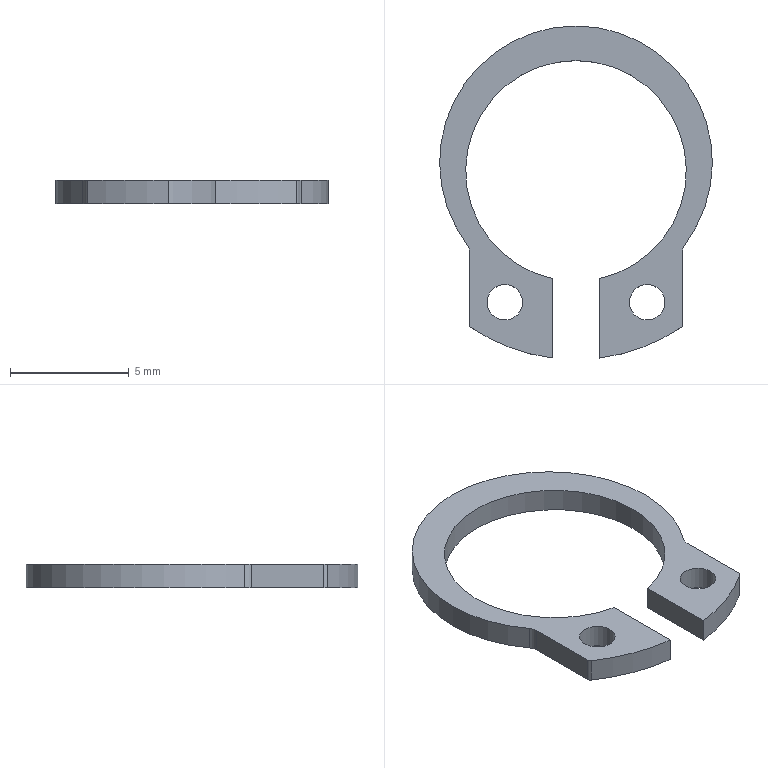Part | NX | features BREP 1, DATUM_CSYS 1 | 1 solid | 16 faces | box 11.5 x 13.997 x 1 mm | volume 50.713 mm3 | cylinder 10 | plane 6 | commonest cylinder face diameters 0.4 x2 1 x2 1.5 x2 15.9 x2 9.3 x1 11.5 x1
STEP:
#1=CARTESIAN_POINT('',(-1.,-4.541,0.));
#2=VERTEX_POINT('',#1);
#3=CARTESIAN_POINT('',(1.,-4.541,0.));
#4=VERTEX_POINT('',#3);
#5=CARTESIAN_POINT('',(0.,0.,0.));
#6=DIRECTION('',(0.,0.,-1.));
#7=DIRECTION('',(-0.2151,-0.9766,0.));
#8=AXIS2_PLACEMENT_3D('',#5,#6,#7);
#9=CIRCLE('',#8,4.65);
#10=EDGE_CURVE('',#2,#4,#9,.T.);
#11=ORIENTED_EDGE('',*,*,#10,.F.);
#12=CARTESIAN_POINT('',(-1.,-7.887,0.));
#13=VERTEX_POINT('',#12);
#14=CARTESIAN_POINT('',(-1.,-7.887,0.));
#15=DIRECTION('',(0.,1.,0.));
#16=VECTOR('',#15,1000.);
#17=LINE('',#14,#16);
#18=EDGE_CURVE('',#13,#2,#17,.T.);
#19=ORIENTED_EDGE('',*,*,#18,.F.);
#20=CARTESIAN_POINT('',(-4.411,-6.614,0.));
#21=VERTEX_POINT('',#20);
#22=CARTESIAN_POINT('',(0.,0.,0.));
#23=DIRECTION('',(0.,0.,1.));
#24=DIRECTION('',(-0.5548,-0.832,0.));
#25=AXIS2_PLACEMENT_3D('',#22,#23,#24);
#26=CIRCLE('',#25,7.95);
#27=EDGE_CURVE('',#21,#13,#26,.T.);
#28=ORIENTED_EDGE('',*,*,#27,.F.);
#29=CARTESIAN_POINT('',(-4.5,-6.448,0.));
#30=VERTEX_POINT('',#29);
#31=CARTESIAN_POINT('',(-4.3,-6.448,0.));
#32=DIRECTION('',(0.,0.,1.));
#33=DIRECTION('',(-1.,0.,0.));
#34=AXIS2_PLACEMENT_3D('',#31,#32,#33);
#35=CIRCLE('',#34,0.2);
#36=EDGE_CURVE('',#30,#21,#35,.T.);
#37=ORIENTED_EDGE('',*,*,#36,.F.);
#38=CARTESIAN_POINT('',(-4.5,-3.39,0.));
#39=VERTEX_POINT('',#38);
#40=CARTESIAN_POINT('',(-4.5,-3.39,0.));
#41=DIRECTION('',(0.,-1.,0.));
#42=VECTOR('',#41,1000.);
#43=LINE('',#40,#42);
#44=EDGE_CURVE('',#39,#30,#43,.T.);
#45=ORIENTED_EDGE('',*,*,#44,.F.);
#46=CARTESIAN_POINT('',(-4.6,-3.09,0.));
#47=VERTEX_POINT('',#46);
#48=CARTESIAN_POINT('',(-5.,-3.39,0.));
#49=DIRECTION('',(0.,0.,-1.));
#50=DIRECTION('',(0.8,0.6,0.));
#51=AXIS2_PLACEMENT_3D('',#48,#49,#50);
#52=CIRCLE('',#51,0.5);
#53=EDGE_CURVE('',#47,#39,#52,.T.);
#54=ORIENTED_EDGE('',*,*,#53,.F.);
#55=CARTESIAN_POINT('',(4.6,-3.09,0.));
#56=VERTEX_POINT('',#55);
#57=CARTESIAN_POINT('',(0.,0.36,0.));
#58=DIRECTION('',(0.,0.,1.));
#59=DIRECTION('',(0.8,-0.6,0.));
#60=AXIS2_PLACEMENT_3D('',#57,#58,#59);
#61=CIRCLE('',#60,5.75);
#62=EDGE_CURVE('',#56,#47,#61,.T.);
#63=ORIENTED_EDGE('',*,*,#62,.F.);
#64=CARTESIAN_POINT('',(4.5,-3.39,0.));
#65=VERTEX_POINT('',#64);
#66=CARTESIAN_POINT('',(5.,-3.39,0.));
#67=DIRECTION('',(0.,0.,-1.));
#68=DIRECTION('',(-1.,0.,0.));
#69=AXIS2_PLACEMENT_3D('',#66,#67,#68);
#70=CIRCLE('',#69,0.5);
#71=EDGE_CURVE('',#65,#56,#70,.T.);
#72=ORIENTED_EDGE('',*,*,#71,.F.);
#73=CARTESIAN_POINT('',(4.5,-6.448,0.));
#74=VERTEX_POINT('',#73);
#75=CARTESIAN_POINT('',(4.5,-6.448,0.));
#76=DIRECTION('',(0.,1.,0.));
#77=VECTOR('',#76,1000.);
#78=LINE('',#75,#77);
#79=EDGE_CURVE('',#74,#65,#78,.T.);
#80=ORIENTED_EDGE('',*,*,#79,.F.);
#81=CARTESIAN_POINT('',(4.411,-6.614,0.));
#82=VERTEX_POINT('',#81);
#83=CARTESIAN_POINT('',(4.3,-6.448,0.));
#84=DIRECTION('',(0.,0.,1.));
#85=DIRECTION('',(0.5548,-0.832,0.));
#86=AXIS2_PLACEMENT_3D('',#83,#84,#85);
#87=CIRCLE('',#86,0.2);
#88=EDGE_CURVE('',#82,#74,#87,.T.);
#89=ORIENTED_EDGE('',*,*,#88,.F.);
#90=CARTESIAN_POINT('',(1.,-7.887,0.));
#91=VERTEX_POINT('',#90);
#92=CARTESIAN_POINT('',(0.,0.,0.));
#93=DIRECTION('',(0.,0.,1.));
#94=DIRECTION('',(0.1258,-0.9921,0.));
#95=AXIS2_PLACEMENT_3D('',#92,#93,#94);
#96=CIRCLE('',#95,7.95);
#97=EDGE_CURVE('',#91,#82,#96,.T.);
#98=ORIENTED_EDGE('',*,*,#97,.F.);
#99=CARTESIAN_POINT('',(1.,-4.541,0.));
#100=DIRECTION('',(0.,-1.,0.));
#101=VECTOR('',#100,1000.);
#102=LINE('',#99,#101);
#103=EDGE_CURVE('',#4,#91,#102,.T.);
#104=ORIENTED_EDGE('',*,*,#103,.F.);
#105=EDGE_LOOP('',(#11,#19,#28,#37,#45,#54,#63,#72,#80,#89,#98,#104));
#106=FACE_BOUND('',#105,.T.);
#107=CARTESIAN_POINT('',(-2.25,-5.54,0.));
#108=VERTEX_POINT('',#107);
#109=CARTESIAN_POINT('',(-3.,-5.54,0.));
#110=DIRECTION('',(0.,0.,-1.));
#111=DIRECTION('',(1.,0.,0.));
#112=AXIS2_PLACEMENT_3D('',#109,#110,#111);
#113=CIRCLE('',#112,0.75);
#114=EDGE_CURVE('',#108,#108,#113,.T.);
#115=ORIENTED_EDGE('',*,*,#114,.F.);
#116=EDGE_LOOP('',(#115));
#117=FACE_BOUND('',#116,.T.);
#118=CARTESIAN_POINT('',(3.75,-5.54,0.));
#119=VERTEX_POINT('',#118);
#120=CARTESIAN_POINT('',(3.,-5.54,0.));
#121=DIRECTION('',(0.,0.,-1.));
#122=DIRECTION('',(1.,0.,0.));
#123=AXIS2_PLACEMENT_3D('',#120,#121,#122);
#124=CIRCLE('',#123,0.75);
#125=EDGE_CURVE('',#119,#119,#124,.T.);
#126=ORIENTED_EDGE('',*,*,#125,.F.);
#127=EDGE_LOOP('',(#126));
#128=FACE_BOUND('',#127,.T.);
#129=CARTESIAN_POINT('',(0.2662,-0.8884,0.));
#130=DIRECTION('',(0.,0.,1.));
#131=DIRECTION('',(-1.,0.,0.));
#132=AXIS2_PLACEMENT_3D('',#129,#130,#131);
#133=PLANE('',#132);
#134=ADVANCED_FACE('',(#106,#117,#128),#133,.F.);
#135=CARTESIAN_POINT('',(1.,-4.541,1.));
#136=VERTEX_POINT('',#135);
#137=CARTESIAN_POINT('',(1.,-7.887,1.));
#138=VERTEX_POINT('',#137);
#139=CARTESIAN_POINT('',(1.,-4.541,1.));
#140=DIRECTION('',(0.,-1.,0.));
#141=VECTOR('',#140,1000.);
#142=LINE('',#139,#141);
#143=EDGE_CURVE('',#136,#138,#142,.T.);
#144=ORIENTED_EDGE('',*,*,#143,.T.);
#145=CARTESIAN_POINT('',(4.411,-6.614,1.));
#146=VERTEX_POINT('',#145);
#147=CARTESIAN_POINT('',(0.,0.,1.));
#148=DIRECTION('',(0.,0.,1.));
#149=DIRECTION('',(0.1258,-0.9921,0.));
#150=AXIS2_PLACEMENT_3D('',#147,#148,#149);
#151=CIRCLE('',#150,7.95);
#152=EDGE_CURVE('',#138,#146,#151,.T.);
#153=ORIENTED_EDGE('',*,*,#152,.T.);
#154=CARTESIAN_POINT('',(4.5,-6.448,1.));
#155=VERTEX_POINT('',#154);
#156=CARTESIAN_POINT('',(4.3,-6.448,1.));
#157=DIRECTION('',(0.,0.,1.));
#158=DIRECTION('',(0.5548,-0.832,0.));
#159=AXIS2_PLACEMENT_3D('',#156,#157,#158);
#160=CIRCLE('',#159,0.2);
#161=EDGE_CURVE('',#146,#155,#160,.T.);
#162=ORIENTED_EDGE('',*,*,#161,.T.);
#163=CARTESIAN_POINT('',(4.5,-3.39,1.));
#164=VERTEX_POINT('',#163);
#165=CARTESIAN_POINT('',(4.5,-6.448,1.));
#166=DIRECTION('',(0.,1.,0.));
#167=VECTOR('',#166,1000.);
#168=LINE('',#165,#167);
#169=EDGE_CURVE('',#155,#164,#168,.T.);
#170=ORIENTED_EDGE('',*,*,#169,.T.);
#171=CARTESIAN_POINT('',(4.6,-3.09,1.));
#172=VERTEX_POINT('',#171);
#173=CARTESIAN_POINT('',(5.,-3.39,1.));
#174=DIRECTION('',(0.,0.,-1.));
#175=DIRECTION('',(-1.,0.,0.));
#176=AXIS2_PLACEMENT_3D('',#173,#174,#175);
#177=CIRCLE('',#176,0.5);
#178=EDGE_CURVE('',#164,#172,#177,.T.);
#179=ORIENTED_EDGE('',*,*,#178,.T.);
#180=CARTESIAN_POINT('',(-4.6,-3.09,1.));
#181=VERTEX_POINT('',#180);
#182=CARTESIAN_POINT('',(0.,0.36,1.));
#183=DIRECTION('',(0.,0.,1.));
#184=DIRECTION('',(0.8,-0.6,0.));
#185=AXIS2_PLACEMENT_3D('',#182,#183,#184);
#186=CIRCLE('',#185,5.75);
#187=EDGE_CURVE('',#172,#181,#186,.T.);
#188=ORIENTED_EDGE('',*,*,#187,.T.);
#189=CARTESIAN_POINT('',(-4.5,-3.39,1.));
#190=VERTEX_POINT('',#189);
#191=CARTESIAN_POINT('',(-5.,-3.39,1.));
#192=DIRECTION('',(0.,0.,-1.));
#193=DIRECTION('',(0.8,0.6,0.));
#194=AXIS2_PLACEMENT_3D('',#191,#192,#193);
#195=CIRCLE('',#194,0.5);
#196=EDGE_CURVE('',#181,#190,#195,.T.);
#197=ORIENTED_EDGE('',*,*,#196,.T.);
#198=CARTESIAN_POINT('',(-4.5,-6.448,1.));
#199=VERTEX_POINT('',#198);
#200=CARTESIAN_POINT('',(-4.5,-3.39,1.));
#201=DIRECTION('',(0.,-1.,0.));
#202=VECTOR('',#201,1000.);
#203=LINE('',#200,#202);
#204=EDGE_CURVE('',#190,#199,#203,.T.);
#205=ORIENTED_EDGE('',*,*,#204,.T.);
#206=CARTESIAN_POINT('',(-4.411,-6.614,1.));
#207=VERTEX_POINT('',#206);
#208=CARTESIAN_POINT('',(-4.3,-6.448,1.));
#209=DIRECTION('',(0.,0.,1.));
#210=DIRECTION('',(-1.,0.,0.));
#211=AXIS2_PLACEMENT_3D('',#208,#209,#210);
#212=CIRCLE('',#211,0.2);
#213=EDGE_CURVE('',#199,#207,#212,.T.);
#214=ORIENTED_EDGE('',*,*,#213,.T.);
#215=CARTESIAN_POINT('',(-1.,-7.887,1.));
#216=VERTEX_POINT('',#215);
#217=CARTESIAN_POINT('',(0.,0.,1.));
#218=DIRECTION('',(0.,0.,1.));
#219=DIRECTION('',(-0.5548,-0.832,0.));
#220=AXIS2_PLACEMENT_3D('',#217,#218,#219);
#221=CIRCLE('',#220,7.95);
#222=EDGE_CURVE('',#207,#216,#221,.T.);
#223=ORIENTED_EDGE('',*,*,#222,.T.);
#224=CARTESIAN_POINT('',(-1.,-4.541,1.));
#225=VERTEX_POINT('',#224);
#226=CARTESIAN_POINT('',(-1.,-7.887,1.));
#227=DIRECTION('',(0.,1.,0.));
#228=VECTOR('',#227,1000.);
#229=LINE('',#226,#228);
#230=EDGE_CURVE('',#216,#225,#229,.T.);
#231=ORIENTED_EDGE('',*,*,#230,.T.);
#232=CARTESIAN_POINT('',(0.,0.,1.));
#233=DIRECTION('',(0.,0.,-1.));
#234=DIRECTION('',(-0.2151,-0.9766,0.));
#235=AXIS2_PLACEMENT_3D('',#232,#233,#234);
#236=CIRCLE('',#235,4.65);
#237=EDGE_CURVE('',#225,#136,#236,.T.);
#238=ORIENTED_EDGE('',*,*,#237,.T.);
#239=EDGE_LOOP('',(#144,#153,#162,#170,#179,#188,#197,#205,#214,#223,#231,#238));
#240=FACE_BOUND('',#239,.T.);
#241=CARTESIAN_POINT('',(-2.25,-5.54,1.));
#242=VERTEX_POINT('',#241);
#243=CARTESIAN_POINT('',(-3.,-5.54,1.));
#244=DIRECTION('',(0.,0.,-1.));
#245=DIRECTION('',(1.,0.,0.));
#246=AXIS2_PLACEMENT_3D('',#243,#244,#245);
#247=CIRCLE('',#246,0.75);
#248=EDGE_CURVE('',#242,#242,#247,.T.);
#249=ORIENTED_EDGE('',*,*,#248,.T.);
#250=EDGE_LOOP('',(#249));
#251=FACE_BOUND('',#250,.T.);
#252=CARTESIAN_POINT('',(3.75,-5.54,1.));
#253=VERTEX_POINT('',#252);
#254=CARTESIAN_POINT('',(3.,-5.54,1.));
#255=DIRECTION('',(0.,0.,-1.));
#256=DIRECTION('',(1.,0.,0.));
#257=AXIS2_PLACEMENT_3D('',#254,#255,#256);
#258=CIRCLE('',#257,0.75);
#259=EDGE_CURVE('',#253,#253,#258,.T.);
#260=ORIENTED_EDGE('',*,*,#259,.T.);
#261=EDGE_LOOP('',(#260));
#262=FACE_BOUND('',#261,.T.);
#263=CARTESIAN_POINT('',(0.2662,-0.8884,1.));
#264=DIRECTION('',(0.,0.,1.));
#265=DIRECTION('',(-1.,0.,0.));
#266=AXIS2_PLACEMENT_3D('',#263,#264,#265);
#267=PLANE('',#266);
#268=ADVANCED_FACE('',(#240,#251,#262),#267,.T.);
#269=ORIENTED_EDGE('',*,*,#103,.T.);
#270=CARTESIAN_POINT('',(1.,-7.887,0.));
#271=DIRECTION('',(0.,0.,1.));
#272=VECTOR('',#271,1000.);
#273=LINE('',#270,#272);
#274=EDGE_CURVE('',#91,#138,#273,.T.);
#275=ORIENTED_EDGE('',*,*,#274,.T.);
#276=ORIENTED_EDGE('',*,*,#143,.F.);
#277=CARTESIAN_POINT('',(1.,-4.541,0.));
#278=DIRECTION('',(0.,0.,1.));
#279=VECTOR('',#278,1000.);
#280=LINE('',#277,#279);
#281=EDGE_CURVE('',#4,#136,#280,.T.);
#282=ORIENTED_EDGE('',*,*,#281,.F.);
#283=EDGE_LOOP('',(#269,#275,#276,#282));
#284=FACE_BOUND('',#283,.T.);
#285=CARTESIAN_POINT('',(1.,-6.214,0.5));
#286=DIRECTION('',(-1.,0.,0.));
#287=DIRECTION('',(0.,1.,0.));
#288=AXIS2_PLACEMENT_3D('',#285,#286,#287);
#289=PLANE('',#288);
#290=ADVANCED_FACE('',(#284),#289,.T.);
#291=ORIENTED_EDGE('',*,*,#97,.T.);
#292=CARTESIAN_POINT('',(4.411,-6.614,0.));
#293=DIRECTION('',(0.,0.,1.));
#294=VECTOR('',#293,1000.);
#295=LINE('',#292,#294);
#296=EDGE_CURVE('',#82,#146,#295,.T.);
#297=ORIENTED_EDGE('',*,*,#296,.T.);
#298=ORIENTED_EDGE('',*,*,#152,.F.);
#299=ORIENTED_EDGE('',*,*,#274,.F.);
#300=EDGE_LOOP('',(#291,#297,#298,#299));
#301=FACE_BOUND('',#300,.T.);
#302=CARTESIAN_POINT('',(0.,0.,0.));
#303=DIRECTION('',(0.,0.,1.));
#304=DIRECTION('',(-0.1258,0.9921,0.));
#305=AXIS2_PLACEMENT_3D('',#302,#303,#304);
#306=CYLINDRICAL_SURFACE('',#305,7.95);
#307=ADVANCED_FACE('',(#301),#306,.T.);
#308=ORIENTED_EDGE('',*,*,#88,.T.);
#309=CARTESIAN_POINT('',(4.5,-6.448,0.));
#310=DIRECTION('',(0.,0.,1.));
#311=VECTOR('',#310,1000.);
#312=LINE('',#309,#311);
#313=EDGE_CURVE('',#74,#155,#312,.T.);
#314=ORIENTED_EDGE('',*,*,#313,.T.);
#315=ORIENTED_EDGE('',*,*,#161,.F.);
#316=ORIENTED_EDGE('',*,*,#296,.F.);
#317=EDGE_LOOP('',(#308,#314,#315,#316));
#318=FACE_BOUND('',#317,.T.);
#319=CARTESIAN_POINT('',(4.3,-6.448,0.));
#320=DIRECTION('',(0.,0.,1.));
#321=DIRECTION('',(-0.5548,0.832,0.));
#322=AXIS2_PLACEMENT_3D('',#319,#320,#321);
#323=CYLINDRICAL_SURFACE('',#322,0.2);
#324=ADVANCED_FACE('',(#318),#323,.T.);
#325=ORIENTED_EDGE('',*,*,#79,.T.);
#326=CARTESIAN_POINT('',(4.5,-3.39,0.));
#327=DIRECTION('',(0.,0.,1.));
#328=VECTOR('',#327,1000.);
#329=LINE('',#326,#328);
#330=EDGE_CURVE('',#65,#164,#329,.T.);
#331=ORIENTED_EDGE('',*,*,#330,.T.);
#332=ORIENTED_EDGE('',*,*,#169,.F.);
#333=ORIENTED_EDGE('',*,*,#313,.F.);
#334=EDGE_LOOP('',(#325,#331,#332,#333));
#335=FACE_BOUND('',#334,.T.);
#336=CARTESIAN_POINT('',(4.5,-4.919,0.5));
#337=DIRECTION('',(1.,0.,0.));
#338=DIRECTION('',(0.,-1.,0.));
#339=AXIS2_PLACEMENT_3D('',#336,#337,#338);
#340=PLANE('',#339);
#341=ADVANCED_FACE('',(#335),#340,.T.);
#342=ORIENTED_EDGE('',*,*,#71,.T.);
#343=CARTESIAN_POINT('',(4.6,-3.09,0.));
#344=DIRECTION('',(0.,0.,1.));
#345=VECTOR('',#344,1000.);
#346=LINE('',#343,#345);
#347=EDGE_CURVE('',#56,#172,#346,.T.);
#348=ORIENTED_EDGE('',*,*,#347,.T.);
#349=ORIENTED_EDGE('',*,*,#178,.F.);
#350=ORIENTED_EDGE('',*,*,#330,.F.);
#351=EDGE_LOOP('',(#342,#348,#349,#350));
#352=FACE_BOUND('',#351,.T.);
#353=CARTESIAN_POINT('',(5.,-3.39,0.));
#354=DIRECTION('',(0.,0.,1.));
#355=DIRECTION('',(1.,0.,0.));
#356=AXIS2_PLACEMENT_3D('',#353,#354,#355);
#357=CYLINDRICAL_SURFACE('',#356,0.5);
#358=ADVANCED_FACE('',(#352),#357,.F.);
#359=ORIENTED_EDGE('',*,*,#347,.F.);
#360=ORIENTED_EDGE('',*,*,#62,.T.);
#361=CARTESIAN_POINT('',(-4.6,-3.09,0.));
#362=DIRECTION('',(0.,0.,1.));
#363=VECTOR('',#362,1000.);
#364=LINE('',#361,#363);
#365=EDGE_CURVE('',#47,#181,#364,.T.);
#366=ORIENTED_EDGE('',*,*,#365,.T.);
#367=ORIENTED_EDGE('',*,*,#187,.F.);
#368=EDGE_LOOP('',(#359,#360,#366,#367));
#369=FACE_BOUND('',#368,.T.);
#370=CARTESIAN_POINT('',(0.,0.36,0.));
#371=DIRECTION('',(0.,0.,1.));
#372=DIRECTION('',(-0.8,0.6,0.));
#373=AXIS2_PLACEMENT_3D('',#370,#371,#372);
#374=CYLINDRICAL_SURFACE('',#373,5.75);
#375=ADVANCED_FACE('',(#369),#374,.T.);
#376=ORIENTED_EDGE('',*,*,#53,.T.);
#377=CARTESIAN_POINT('',(-4.5,-3.39,0.));
#378=DIRECTION('',(0.,0.,1.));
#379=VECTOR('',#378,1000.);
#380=LINE('',#377,#379);
#381=EDGE_CURVE('',#39,#190,#380,.T.);
#382=ORIENTED_EDGE('',*,*,#381,.T.);
#383=ORIENTED_EDGE('',*,*,#196,.F.);
#384=ORIENTED_EDGE('',*,*,#365,.F.);
#385=EDGE_LOOP('',(#376,#382,#383,#384));
#386=FACE_BOUND('',#385,.T.);
#387=CARTESIAN_POINT('',(-5.,-3.39,0.));
#388=DIRECTION('',(0.,0.,1.));
#389=DIRECTION('',(-0.8,-0.6,0.));
#390=AXIS2_PLACEMENT_3D('',#387,#388,#389);
#391=CYLINDRICAL_SURFACE('',#390,0.5);
#392=ADVANCED_FACE('',(#386),#391,.F.);
#393=ORIENTED_EDGE('',*,*,#44,.T.);
#394=CARTESIAN_POINT('',(-4.5,-6.448,0.));
#395=DIRECTION('',(0.,0.,1.));
#396=VECTOR('',#395,1000.);
#397=LINE('',#394,#396);
#398=EDGE_CURVE('',#30,#199,#397,.T.);
#399=ORIENTED_EDGE('',*,*,#398,.T.);
#400=ORIENTED_EDGE('',*,*,#204,.F.);
#401=ORIENTED_EDGE('',*,*,#381,.F.);
#402=EDGE_LOOP('',(#393,#399,#400,#401));
#403=FACE_BOUND('',#402,.T.);
#404=CARTESIAN_POINT('',(-4.5,-4.919,0.5));
#405=DIRECTION('',(-1.,0.,0.));
#406=DIRECTION('',(0.,1.,0.));
#407=AXIS2_PLACEMENT_3D('',#404,#405,#406);
#408=PLANE('',#407);
#409=ADVANCED_FACE('',(#403),#408,.T.);
#410=ORIENTED_EDGE('',*,*,#36,.T.);
#411=CARTESIAN_POINT('',(-4.411,-6.614,0.));
#412=DIRECTION('',(0.,0.,1.));
#413=VECTOR('',#412,1000.);
#414=LINE('',#411,#413);
#415=EDGE_CURVE('',#21,#207,#414,.T.);
#416=ORIENTED_EDGE('',*,*,#415,.T.);
#417=ORIENTED_EDGE('',*,*,#213,.F.);
#418=ORIENTED_EDGE('',*,*,#398,.F.);
#419=EDGE_LOOP('',(#410,#416,#417,#418));
#420=FACE_BOUND('',#419,.T.);
#421=CARTESIAN_POINT('',(-4.3,-6.448,0.));
#422=DIRECTION('',(0.,0.,1.));
#423=DIRECTION('',(1.,0.,0.));
#424=AXIS2_PLACEMENT_3D('',#421,#422,#423);
#425=CYLINDRICAL_SURFACE('',#424,0.2);
#426=ADVANCED_FACE('',(#420),#425,.T.);
#427=ORIENTED_EDGE('',*,*,#27,.T.);
#428=CARTESIAN_POINT('',(-1.,-7.887,0.));
#429=DIRECTION('',(0.,0.,1.));
#430=VECTOR('',#429,1000.);
#431=LINE('',#428,#430);
#432=EDGE_CURVE('',#13,#216,#431,.T.);
#433=ORIENTED_EDGE('',*,*,#432,.T.);
#434=ORIENTED_EDGE('',*,*,#222,.F.);
#435=ORIENTED_EDGE('',*,*,#415,.F.);
#436=EDGE_LOOP('',(#427,#433,#434,#435));
#437=FACE_BOUND('',#436,.T.);
#438=CARTESIAN_POINT('',(0.,0.,0.));
#439=DIRECTION('',(0.,0.,1.));
#440=DIRECTION('',(0.5548,0.832,0.));
#441=AXIS2_PLACEMENT_3D('',#438,#439,#440);
#442=CYLINDRICAL_SURFACE('',#441,7.95);
#443=ADVANCED_FACE('',(#437),#442,.T.);
#444=ORIENTED_EDGE('',*,*,#18,.T.);
#445=CARTESIAN_POINT('',(-1.,-4.541,0.));
#446=DIRECTION('',(0.,0.,1.));
#447=VECTOR('',#446,1000.);
#448=LINE('',#445,#447);
#449=EDGE_CURVE('',#2,#225,#448,.T.);
#450=ORIENTED_EDGE('',*,*,#449,.T.);
#451=ORIENTED_EDGE('',*,*,#230,.F.);
#452=ORIENTED_EDGE('',*,*,#432,.F.);
#453=EDGE_LOOP('',(#444,#450,#451,#452));
#454=FACE_BOUND('',#453,.T.);
#455=CARTESIAN_POINT('',(-1.,-6.214,0.5));
#456=DIRECTION('',(1.,0.,0.));
#457=DIRECTION('',(0.,-1.,0.));
#458=AXIS2_PLACEMENT_3D('',#455,#456,#457);
#459=PLANE('',#458);
#460=ADVANCED_FACE('',(#454),#459,.T.);
#461=ORIENTED_EDGE('',*,*,#10,.T.);
#462=ORIENTED_EDGE('',*,*,#281,.T.);
#463=ORIENTED_EDGE('',*,*,#237,.F.);
#464=ORIENTED_EDGE('',*,*,#449,.F.);
#465=EDGE_LOOP('',(#461,#462,#463,#464));
#466=FACE_BOUND('',#465,.T.);
#467=CARTESIAN_POINT('',(0.,0.,0.));
#468=DIRECTION('',(0.,0.,1.));
#469=DIRECTION('',(-0.2151,0.9766,0.));
#470=AXIS2_PLACEMENT_3D('',#467,#468,#469);
#471=CYLINDRICAL_SURFACE('',#470,4.65);
#472=ADVANCED_FACE('',(#466),#471,.F.);
#473=ORIENTED_EDGE('',*,*,#114,.T.);
#474=CARTESIAN_POINT('',(-2.25,-5.54,0.));
#475=DIRECTION('',(0.,0.,1.));
#476=VECTOR('',#475,1000.);
#477=LINE('',#474,#476);
#478=EDGE_CURVE('',#108,#242,#477,.T.);
#479=ORIENTED_EDGE('',*,*,#478,.T.);
#480=ORIENTED_EDGE('',*,*,#248,.F.);
#481=ORIENTED_EDGE('',*,*,#478,.F.);
#482=EDGE_LOOP('',(#473,#479,#480,#481));
#483=FACE_BOUND('',#482,.T.);
#484=CARTESIAN_POINT('',(-3.,-5.54,0.));
#485=DIRECTION('',(0.,0.,1.));
#486=DIRECTION('',(-1.,0.,0.));
#487=AXIS2_PLACEMENT_3D('',#484,#485,#486);
#488=CYLINDRICAL_SURFACE('',#487,0.75);
#489=ADVANCED_FACE('',(#483),#488,.F.);
#490=ORIENTED_EDGE('',*,*,#125,.T.);
#491=CARTESIAN_POINT('',(3.75,-5.54,0.));
#492=DIRECTION('',(0.,0.,1.));
#493=VECTOR('',#492,1000.);
#494=LINE('',#491,#493);
#495=EDGE_CURVE('',#119,#253,#494,.T.);
#496=ORIENTED_EDGE('',*,*,#495,.T.);
#497=ORIENTED_EDGE('',*,*,#259,.F.);
#498=ORIENTED_EDGE('',*,*,#495,.F.);
#499=EDGE_LOOP('',(#490,#496,#497,#498));
#500=FACE_BOUND('',#499,.T.);
#501=CARTESIAN_POINT('',(3.,-5.54,0.));
#502=DIRECTION('',(0.,0.,1.));
#503=DIRECTION('',(-1.,0.,0.));
#504=AXIS2_PLACEMENT_3D('',#501,#502,#503);
#505=CYLINDRICAL_SURFACE('',#504,0.75);
#506=ADVANCED_FACE('',(#500),#505,.F.);
#507=CLOSED_SHELL('',(#134,#268,#290,#307,#324,#341,#358,#375,#392,#409,#426,#443,#460,#472,#489,#506));
#508=MANIFOLD_SOLID_BREP('',#507);
#509=(LENGTH_UNIT()NAMED_UNIT(*)SI_UNIT(.MILLI.,.METRE.));
#510=UNCERTAINTY_MEASURE_WITH_UNIT(LENGTH_MEASURE(0.00001),#509,'','');
#511=(NAMED_UNIT(*)PLANE_ANGLE_UNIT()SI_UNIT($,.RADIAN.));
#512=(NAMED_UNIT(*)SI_UNIT($,.STERADIAN.)SOLID_ANGLE_UNIT());
#513=(GEOMETRIC_REPRESENTATION_CONTEXT(3)GLOBAL_UNCERTAINTY_ASSIGNED_CONTEXT((#510))GLOBAL_UNIT_ASSIGNED_CONTEXT((#509,#511,#512))REPRESENTATION_CONTEXT('',''));
#514=ADVANCED_BREP_SHAPE_REPRESENTATION('',(#508),#513);